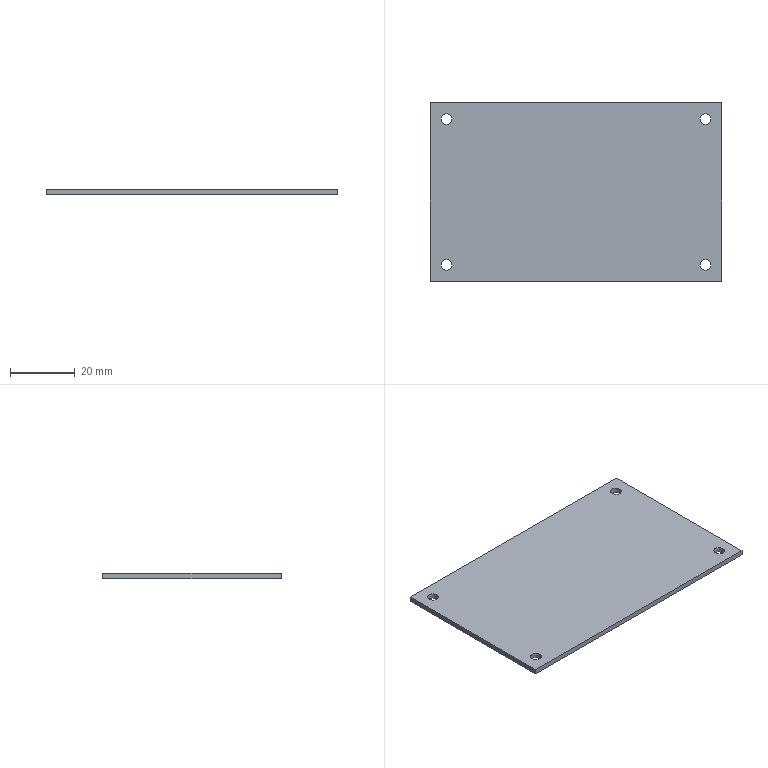Part | SolidWorks | features Extrusion 1 | 1 solid | 14 faces | box 90 x 55 x 1.6 mm | volume 7865 mm3 | cylinder 8 | plane 6 | commonest cylinder face diameters 3.3 x8
STEP:
#1=CARTESIAN_POINT('',(38.35,22.5,-0.8));
#2=VERTEX_POINT('',#1);
#3=CARTESIAN_POINT('',(41.65,22.5,-0.8));
#4=VERTEX_POINT('',#3);
#5=CARTESIAN_POINT('',(40.,22.5,-0.8));
#6=DIRECTION('',(0.,0.,1.));
#7=DIRECTION('',(1.,0.,0.));
#8=AXIS2_PLACEMENT_3D('',#5,#6,#7);
#9=CIRCLE('',#8,1.65);
#10=EDGE_CURVE('',#2,#4,#9,.T.);
#11=ORIENTED_EDGE('',*,*,#10,.F.);
#12=CARTESIAN_POINT('',(38.35,22.5,0.8));
#13=VERTEX_POINT('',#12);
#14=CARTESIAN_POINT('',(38.35,22.5,-0.8));
#15=DIRECTION('',(0.,0.,1.));
#16=VECTOR('',#15,1000.);
#17=LINE('',#14,#16);
#18=EDGE_CURVE('',#2,#13,#17,.T.);
#19=ORIENTED_EDGE('',*,*,#18,.T.);
#20=CARTESIAN_POINT('',(41.65,22.5,0.8));
#21=VERTEX_POINT('',#20);
#22=CARTESIAN_POINT('',(40.,22.5,0.8));
#23=DIRECTION('',(0.,0.,1.));
#24=DIRECTION('',(1.,0.,0.));
#25=AXIS2_PLACEMENT_3D('',#22,#23,#24);
#26=CIRCLE('',#25,1.65);
#27=EDGE_CURVE('',#13,#21,#26,.T.);
#28=ORIENTED_EDGE('',*,*,#27,.T.);
#29=CARTESIAN_POINT('',(41.65,22.5,-0.8));
#30=DIRECTION('',(0.,0.,1.));
#31=VECTOR('',#30,1000.);
#32=LINE('',#29,#31);
#33=EDGE_CURVE('',#4,#21,#32,.T.);
#34=ORIENTED_EDGE('',*,*,#33,.F.);
#35=EDGE_LOOP('',(#11,#19,#28,#34));
#36=FACE_OUTER_BOUND('',#35,.T.);
#37=CARTESIAN_POINT('',(40.,22.5,-0.8));
#38=DIRECTION('',(0.,0.,1.));
#39=DIRECTION('',(1.,0.,0.));
#40=AXIS2_PLACEMENT_3D('',#37,#38,#39);
#41=CYLINDRICAL_SURFACE('',#40,1.65);
#42=ADVANCED_FACE('',(#36),#41,.F.);
#43=CARTESIAN_POINT('',(38.35,-22.5,-0.8));
#44=VERTEX_POINT('',#43);
#45=CARTESIAN_POINT('',(41.65,-22.5,-0.8));
#46=VERTEX_POINT('',#45);
#47=CARTESIAN_POINT('',(40.,-22.5,-0.8));
#48=DIRECTION('',(0.,0.,1.));
#49=DIRECTION('',(1.,0.,0.));
#50=AXIS2_PLACEMENT_3D('',#47,#48,#49);
#51=CIRCLE('',#50,1.65);
#52=EDGE_CURVE('',#44,#46,#51,.T.);
#53=ORIENTED_EDGE('',*,*,#52,.F.);
#54=CARTESIAN_POINT('',(38.35,-22.5,0.8));
#55=VERTEX_POINT('',#54);
#56=CARTESIAN_POINT('',(38.35,-22.5,-0.8));
#57=DIRECTION('',(0.,0.,1.));
#58=VECTOR('',#57,1000.);
#59=LINE('',#56,#58);
#60=EDGE_CURVE('',#44,#55,#59,.T.);
#61=ORIENTED_EDGE('',*,*,#60,.T.);
#62=CARTESIAN_POINT('',(41.65,-22.5,0.8));
#63=VERTEX_POINT('',#62);
#64=CARTESIAN_POINT('',(40.,-22.5,0.8));
#65=DIRECTION('',(0.,0.,1.));
#66=DIRECTION('',(1.,0.,0.));
#67=AXIS2_PLACEMENT_3D('',#64,#65,#66);
#68=CIRCLE('',#67,1.65);
#69=EDGE_CURVE('',#55,#63,#68,.T.);
#70=ORIENTED_EDGE('',*,*,#69,.T.);
#71=CARTESIAN_POINT('',(41.65,-22.5,-0.8));
#72=DIRECTION('',(0.,0.,1.));
#73=VECTOR('',#72,1000.);
#74=LINE('',#71,#73);
#75=EDGE_CURVE('',#46,#63,#74,.T.);
#76=ORIENTED_EDGE('',*,*,#75,.F.);
#77=EDGE_LOOP('',(#53,#61,#70,#76));
#78=FACE_OUTER_BOUND('',#77,.T.);
#79=CARTESIAN_POINT('',(40.,-22.5,-0.8));
#80=DIRECTION('',(0.,0.,1.));
#81=DIRECTION('',(1.,0.,0.));
#82=AXIS2_PLACEMENT_3D('',#79,#80,#81);
#83=CYLINDRICAL_SURFACE('',#82,1.65);
#84=ADVANCED_FACE('',(#78),#83,.F.);
#85=CARTESIAN_POINT('',(-41.65,22.5,-0.8));
#86=VERTEX_POINT('',#85);
#87=CARTESIAN_POINT('',(-38.35,22.5,-0.8));
#88=VERTEX_POINT('',#87);
#89=CARTESIAN_POINT('',(-40.,22.5,-0.8));
#90=DIRECTION('',(0.,0.,1.));
#91=DIRECTION('',(1.,0.,0.));
#92=AXIS2_PLACEMENT_3D('',#89,#90,#91);
#93=CIRCLE('',#92,1.65);
#94=EDGE_CURVE('',#86,#88,#93,.T.);
#95=ORIENTED_EDGE('',*,*,#94,.F.);
#96=CARTESIAN_POINT('',(-41.65,22.5,0.8));
#97=VERTEX_POINT('',#96);
#98=CARTESIAN_POINT('',(-41.65,22.5,-0.8));
#99=DIRECTION('',(0.,0.,1.));
#100=VECTOR('',#99,1000.);
#101=LINE('',#98,#100);
#102=EDGE_CURVE('',#86,#97,#101,.T.);
#103=ORIENTED_EDGE('',*,*,#102,.T.);
#104=CARTESIAN_POINT('',(-38.35,22.5,0.8));
#105=VERTEX_POINT('',#104);
#106=CARTESIAN_POINT('',(-40.,22.5,0.8));
#107=DIRECTION('',(0.,0.,1.));
#108=DIRECTION('',(1.,0.,0.));
#109=AXIS2_PLACEMENT_3D('',#106,#107,#108);
#110=CIRCLE('',#109,1.65);
#111=EDGE_CURVE('',#97,#105,#110,.T.);
#112=ORIENTED_EDGE('',*,*,#111,.T.);
#113=CARTESIAN_POINT('',(-38.35,22.5,-0.8));
#114=DIRECTION('',(0.,0.,1.));
#115=VECTOR('',#114,1000.);
#116=LINE('',#113,#115);
#117=EDGE_CURVE('',#88,#105,#116,.T.);
#118=ORIENTED_EDGE('',*,*,#117,.F.);
#119=EDGE_LOOP('',(#95,#103,#112,#118));
#120=FACE_OUTER_BOUND('',#119,.T.);
#121=CARTESIAN_POINT('',(-40.,22.5,-0.8));
#122=DIRECTION('',(0.,0.,1.));
#123=DIRECTION('',(1.,0.,0.));
#124=AXIS2_PLACEMENT_3D('',#121,#122,#123);
#125=CYLINDRICAL_SURFACE('',#124,1.65);
#126=ADVANCED_FACE('',(#120),#125,.F.);
#127=CARTESIAN_POINT('',(-41.65,-22.5,-0.8));
#128=VERTEX_POINT('',#127);
#129=CARTESIAN_POINT('',(-38.35,-22.5,-0.8));
#130=VERTEX_POINT('',#129);
#131=CARTESIAN_POINT('',(-40.,-22.5,-0.8));
#132=DIRECTION('',(0.,0.,1.));
#133=DIRECTION('',(1.,0.,0.));
#134=AXIS2_PLACEMENT_3D('',#131,#132,#133);
#135=CIRCLE('',#134,1.65);
#136=EDGE_CURVE('',#128,#130,#135,.T.);
#137=ORIENTED_EDGE('',*,*,#136,.F.);
#138=CARTESIAN_POINT('',(-41.65,-22.5,0.8));
#139=VERTEX_POINT('',#138);
#140=CARTESIAN_POINT('',(-41.65,-22.5,-0.8));
#141=DIRECTION('',(0.,0.,1.));
#142=VECTOR('',#141,1000.);
#143=LINE('',#140,#142);
#144=EDGE_CURVE('',#128,#139,#143,.T.);
#145=ORIENTED_EDGE('',*,*,#144,.T.);
#146=CARTESIAN_POINT('',(-38.35,-22.5,0.8));
#147=VERTEX_POINT('',#146);
#148=CARTESIAN_POINT('',(-40.,-22.5,0.8));
#149=DIRECTION('',(0.,0.,1.));
#150=DIRECTION('',(1.,0.,0.));
#151=AXIS2_PLACEMENT_3D('',#148,#149,#150);
#152=CIRCLE('',#151,1.65);
#153=EDGE_CURVE('',#139,#147,#152,.T.);
#154=ORIENTED_EDGE('',*,*,#153,.T.);
#155=CARTESIAN_POINT('',(-38.35,-22.5,-0.8));
#156=DIRECTION('',(0.,0.,1.));
#157=VECTOR('',#156,1000.);
#158=LINE('',#155,#157);
#159=EDGE_CURVE('',#130,#147,#158,.T.);
#160=ORIENTED_EDGE('',*,*,#159,.F.);
#161=EDGE_LOOP('',(#137,#145,#154,#160));
#162=FACE_OUTER_BOUND('',#161,.T.);
#163=CARTESIAN_POINT('',(-40.,-22.5,-0.8));
#164=DIRECTION('',(0.,0.,1.));
#165=DIRECTION('',(1.,0.,0.));
#166=AXIS2_PLACEMENT_3D('',#163,#164,#165);
#167=CYLINDRICAL_SURFACE('',#166,1.65);
#168=ADVANCED_FACE('',(#162),#167,.F.);
#169=CARTESIAN_POINT('',(-45.,27.5,0.8));
#170=VERTEX_POINT('',#169);
#171=CARTESIAN_POINT('',(-45.,-27.5,0.8));
#172=VERTEX_POINT('',#171);
#173=CARTESIAN_POINT('',(-45.,27.5,0.8));
#174=DIRECTION('',(0.,-1.,0.));
#175=VECTOR('',#174,1000.);
#176=LINE('',#173,#175);
#177=EDGE_CURVE('',#170,#172,#176,.T.);
#178=ORIENTED_EDGE('',*,*,#177,.F.);
#179=CARTESIAN_POINT('',(-45.,27.5,-0.8));
#180=VERTEX_POINT('',#179);
#181=CARTESIAN_POINT('',(-45.,27.5,-0.8));
#182=DIRECTION('',(0.,0.,1.));
#183=VECTOR('',#182,1000.);
#184=LINE('',#181,#183);
#185=EDGE_CURVE('',#180,#170,#184,.T.);
#186=ORIENTED_EDGE('',*,*,#185,.F.);
#187=CARTESIAN_POINT('',(-45.,-27.5,-0.8));
#188=VERTEX_POINT('',#187);
#189=CARTESIAN_POINT('',(-45.,27.5,-0.8));
#190=DIRECTION('',(0.,-1.,0.));
#191=VECTOR('',#190,1000.);
#192=LINE('',#189,#191);
#193=EDGE_CURVE('',#180,#188,#192,.T.);
#194=ORIENTED_EDGE('',*,*,#193,.T.);
#195=CARTESIAN_POINT('',(-45.,-27.5,-0.8));
#196=DIRECTION('',(0.,0.,1.));
#197=VECTOR('',#196,1000.);
#198=LINE('',#195,#197);
#199=EDGE_CURVE('',#188,#172,#198,.T.);
#200=ORIENTED_EDGE('',*,*,#199,.T.);
#201=EDGE_LOOP('',(#178,#186,#194,#200));
#202=FACE_OUTER_BOUND('',#201,.T.);
#203=CARTESIAN_POINT('',(-45.,27.5,-0.8));
#204=DIRECTION('',(-1.,0.,0.));
#205=DIRECTION('',(0.,0.,1.));
#206=AXIS2_PLACEMENT_3D('',#203,#204,#205);
#207=PLANE('',#206);
#208=ADVANCED_FACE('',(#202),#207,.T.);
#209=CARTESIAN_POINT('',(45.,27.5,0.8));
#210=VERTEX_POINT('',#209);
#211=CARTESIAN_POINT('',(45.,27.5,0.8));
#212=DIRECTION('',(-1.,0.,0.));
#213=VECTOR('',#212,1000.);
#214=LINE('',#211,#213);
#215=EDGE_CURVE('',#210,#170,#214,.T.);
#216=ORIENTED_EDGE('',*,*,#215,.F.);
#217=CARTESIAN_POINT('',(45.,27.5,-0.8));
#218=VERTEX_POINT('',#217);
#219=CARTESIAN_POINT('',(45.,27.5,-0.8));
#220=DIRECTION('',(0.,0.,1.));
#221=VECTOR('',#220,1000.);
#222=LINE('',#219,#221);
#223=EDGE_CURVE('',#218,#210,#222,.T.);
#224=ORIENTED_EDGE('',*,*,#223,.F.);
#225=CARTESIAN_POINT('',(45.,27.5,-0.8));
#226=DIRECTION('',(-1.,0.,0.));
#227=VECTOR('',#226,1000.);
#228=LINE('',#225,#227);
#229=EDGE_CURVE('',#218,#180,#228,.T.);
#230=ORIENTED_EDGE('',*,*,#229,.T.);
#231=ORIENTED_EDGE('',*,*,#185,.T.);
#232=EDGE_LOOP('',(#216,#224,#230,#231));
#233=FACE_OUTER_BOUND('',#232,.T.);
#234=CARTESIAN_POINT('',(45.,27.5,-0.8));
#235=DIRECTION('',(0.,1.,0.));
#236=DIRECTION('',(0.,0.,1.));
#237=AXIS2_PLACEMENT_3D('',#234,#235,#236);
#238=PLANE('',#237);
#239=ADVANCED_FACE('',(#233),#238,.T.);
#240=CARTESIAN_POINT('',(45.,-27.5,0.8));
#241=VERTEX_POINT('',#240);
#242=CARTESIAN_POINT('',(45.,-27.5,0.8));
#243=DIRECTION('',(0.,1.,0.));
#244=VECTOR('',#243,1000.);
#245=LINE('',#242,#244);
#246=EDGE_CURVE('',#241,#210,#245,.T.);
#247=ORIENTED_EDGE('',*,*,#246,.F.);
#248=CARTESIAN_POINT('',(45.,-27.5,-0.8));
#249=VERTEX_POINT('',#248);
#250=CARTESIAN_POINT('',(45.,-27.5,-0.8));
#251=DIRECTION('',(0.,0.,1.));
#252=VECTOR('',#251,1000.);
#253=LINE('',#250,#252);
#254=EDGE_CURVE('',#249,#241,#253,.T.);
#255=ORIENTED_EDGE('',*,*,#254,.F.);
#256=CARTESIAN_POINT('',(45.,-27.5,-0.8));
#257=DIRECTION('',(0.,1.,0.));
#258=VECTOR('',#257,1000.);
#259=LINE('',#256,#258);
#260=EDGE_CURVE('',#249,#218,#259,.T.);
#261=ORIENTED_EDGE('',*,*,#260,.T.);
#262=ORIENTED_EDGE('',*,*,#223,.T.);
#263=EDGE_LOOP('',(#247,#255,#261,#262));
#264=FACE_OUTER_BOUND('',#263,.T.);
#265=CARTESIAN_POINT('',(45.,-27.5,-0.8));
#266=DIRECTION('',(1.,0.,0.));
#267=DIRECTION('',(0.,0.,-1.));
#268=AXIS2_PLACEMENT_3D('',#265,#266,#267);
#269=PLANE('',#268);
#270=ADVANCED_FACE('',(#264),#269,.T.);
#271=CARTESIAN_POINT('',(-45.,-27.5,0.8));
#272=DIRECTION('',(1.,0.,0.));
#273=VECTOR('',#272,1000.);
#274=LINE('',#271,#273);
#275=EDGE_CURVE('',#172,#241,#274,.T.);
#276=ORIENTED_EDGE('',*,*,#275,.F.);
#277=ORIENTED_EDGE('',*,*,#199,.F.);
#278=CARTESIAN_POINT('',(-45.,-27.5,-0.8));
#279=DIRECTION('',(1.,0.,0.));
#280=VECTOR('',#279,1000.);
#281=LINE('',#278,#280);
#282=EDGE_CURVE('',#188,#249,#281,.T.);
#283=ORIENTED_EDGE('',*,*,#282,.T.);
#284=ORIENTED_EDGE('',*,*,#254,.T.);
#285=EDGE_LOOP('',(#276,#277,#283,#284));
#286=FACE_OUTER_BOUND('',#285,.T.);
#287=CARTESIAN_POINT('',(-45.,-27.5,-0.8));
#288=DIRECTION('',(0.,-1.,0.));
#289=DIRECTION('',(0.,0.,-1.));
#290=AXIS2_PLACEMENT_3D('',#287,#288,#289);
#291=PLANE('',#290);
#292=ADVANCED_FACE('',(#286),#291,.T.);
#293=CARTESIAN_POINT('',(40.,22.5,-0.8));
#294=DIRECTION('',(0.,0.,1.));
#295=DIRECTION('',(1.,0.,0.));
#296=AXIS2_PLACEMENT_3D('',#293,#294,#295);
#297=CIRCLE('',#296,1.65);
#298=EDGE_CURVE('',#4,#2,#297,.T.);
#299=ORIENTED_EDGE('',*,*,#298,.T.);
#300=ORIENTED_EDGE('',*,*,#10,.T.);
#301=EDGE_LOOP('',(#299,#300));
#302=FACE_BOUND('',#301,.T.);
#303=CARTESIAN_POINT('',(40.,-22.5,-0.8));
#304=DIRECTION('',(0.,0.,1.));
#305=DIRECTION('',(1.,0.,0.));
#306=AXIS2_PLACEMENT_3D('',#303,#304,#305);
#307=CIRCLE('',#306,1.65);
#308=EDGE_CURVE('',#46,#44,#307,.T.);
#309=ORIENTED_EDGE('',*,*,#308,.T.);
#310=ORIENTED_EDGE('',*,*,#52,.T.);
#311=EDGE_LOOP('',(#309,#310));
#312=FACE_BOUND('',#311,.T.);
#313=CARTESIAN_POINT('',(-40.,22.5,-0.8));
#314=DIRECTION('',(0.,0.,1.));
#315=DIRECTION('',(1.,0.,0.));
#316=AXIS2_PLACEMENT_3D('',#313,#314,#315);
#317=CIRCLE('',#316,1.65);
#318=EDGE_CURVE('',#88,#86,#317,.T.);
#319=ORIENTED_EDGE('',*,*,#318,.T.);
#320=ORIENTED_EDGE('',*,*,#94,.T.);
#321=EDGE_LOOP('',(#319,#320));
#322=FACE_BOUND('',#321,.T.);
#323=CARTESIAN_POINT('',(-40.,-22.5,-0.8));
#324=DIRECTION('',(0.,0.,1.));
#325=DIRECTION('',(1.,0.,0.));
#326=AXIS2_PLACEMENT_3D('',#323,#324,#325);
#327=CIRCLE('',#326,1.65);
#328=EDGE_CURVE('',#130,#128,#327,.T.);
#329=ORIENTED_EDGE('',*,*,#328,.T.);
#330=ORIENTED_EDGE('',*,*,#136,.T.);
#331=EDGE_LOOP('',(#329,#330));
#332=FACE_BOUND('',#331,.T.);
#333=ORIENTED_EDGE('',*,*,#193,.F.);
#334=ORIENTED_EDGE('',*,*,#229,.F.);
#335=ORIENTED_EDGE('',*,*,#260,.F.);
#336=ORIENTED_EDGE('',*,*,#282,.F.);
#337=EDGE_LOOP('',(#333,#334,#335,#336));
#338=FACE_OUTER_BOUND('',#337,.T.);
#339=CARTESIAN_POINT('',(0.,0.,-0.8));
#340=DIRECTION('',(0.,0.,1.));
#341=DIRECTION('',(1.,0.,0.));
#342=AXIS2_PLACEMENT_3D('',#339,#340,#341);
#343=PLANE('',#342);
#344=ADVANCED_FACE('',(#302,#312,#322,#332,#338),#343,.F.);
#345=CARTESIAN_POINT('',(40.,22.5,0.8));
#346=DIRECTION('',(0.,0.,1.));
#347=DIRECTION('',(1.,0.,0.));
#348=AXIS2_PLACEMENT_3D('',#345,#346,#347);
#349=CIRCLE('',#348,1.65);
#350=EDGE_CURVE('',#21,#13,#349,.T.);
#351=ORIENTED_EDGE('',*,*,#350,.F.);
#352=ORIENTED_EDGE('',*,*,#27,.F.);
#353=EDGE_LOOP('',(#351,#352));
#354=FACE_BOUND('',#353,.T.);
#355=CARTESIAN_POINT('',(40.,-22.5,0.8));
#356=DIRECTION('',(0.,0.,1.));
#357=DIRECTION('',(1.,0.,0.));
#358=AXIS2_PLACEMENT_3D('',#355,#356,#357);
#359=CIRCLE('',#358,1.65);
#360=EDGE_CURVE('',#63,#55,#359,.T.);
#361=ORIENTED_EDGE('',*,*,#360,.F.);
#362=ORIENTED_EDGE('',*,*,#69,.F.);
#363=EDGE_LOOP('',(#361,#362));
#364=FACE_BOUND('',#363,.T.);
#365=CARTESIAN_POINT('',(-40.,22.5,0.8));
#366=DIRECTION('',(0.,0.,1.));
#367=DIRECTION('',(1.,0.,0.));
#368=AXIS2_PLACEMENT_3D('',#365,#366,#367);
#369=CIRCLE('',#368,1.65);
#370=EDGE_CURVE('',#105,#97,#369,.T.);
#371=ORIENTED_EDGE('',*,*,#370,.F.);
#372=ORIENTED_EDGE('',*,*,#111,.F.);
#373=EDGE_LOOP('',(#371,#372));
#374=FACE_BOUND('',#373,.T.);
#375=CARTESIAN_POINT('',(-40.,-22.5,0.8));
#376=DIRECTION('',(0.,0.,1.));
#377=DIRECTION('',(1.,0.,0.));
#378=AXIS2_PLACEMENT_3D('',#375,#376,#377);
#379=CIRCLE('',#378,1.65);
#380=EDGE_CURVE('',#147,#139,#379,.T.);
#381=ORIENTED_EDGE('',*,*,#380,.F.);
#382=ORIENTED_EDGE('',*,*,#153,.F.);
#383=EDGE_LOOP('',(#381,#382));
#384=FACE_BOUND('',#383,.T.);
#385=ORIENTED_EDGE('',*,*,#177,.T.);
#386=ORIENTED_EDGE('',*,*,#275,.T.);
#387=ORIENTED_EDGE('',*,*,#246,.T.);
#388=ORIENTED_EDGE('',*,*,#215,.T.);
#389=EDGE_LOOP('',(#385,#386,#387,#388));
#390=FACE_OUTER_BOUND('',#389,.T.);
#391=CARTESIAN_POINT('',(0.,0.,0.8));
#392=DIRECTION('',(0.,0.,1.));
#393=DIRECTION('',(1.,0.,0.));
#394=AXIS2_PLACEMENT_3D('',#391,#392,#393);
#395=PLANE('',#394);
#396=ADVANCED_FACE('',(#354,#364,#374,#384,#390),#395,.T.);
#397=ORIENTED_EDGE('',*,*,#144,.F.);
#398=ORIENTED_EDGE('',*,*,#328,.F.);
#399=ORIENTED_EDGE('',*,*,#159,.T.);
#400=ORIENTED_EDGE('',*,*,#380,.T.);
#401=EDGE_LOOP('',(#397,#398,#399,#400));
#402=FACE_OUTER_BOUND('',#401,.T.);
#403=CARTESIAN_POINT('',(-40.,-22.5,-0.8));
#404=DIRECTION('',(0.,0.,1.));
#405=DIRECTION('',(1.,0.,0.));
#406=AXIS2_PLACEMENT_3D('',#403,#404,#405);
#407=CYLINDRICAL_SURFACE('',#406,1.65);
#408=ADVANCED_FACE('',(#402),#407,.F.);
#409=ORIENTED_EDGE('',*,*,#102,.F.);
#410=ORIENTED_EDGE('',*,*,#318,.F.);
#411=ORIENTED_EDGE('',*,*,#117,.T.);
#412=ORIENTED_EDGE('',*,*,#370,.T.);
#413=EDGE_LOOP('',(#409,#410,#411,#412));
#414=FACE_OUTER_BOUND('',#413,.T.);
#415=CARTESIAN_POINT('',(-40.,22.5,-0.8));
#416=DIRECTION('',(0.,0.,1.));
#417=DIRECTION('',(1.,0.,0.));
#418=AXIS2_PLACEMENT_3D('',#415,#416,#417);
#419=CYLINDRICAL_SURFACE('',#418,1.65);
#420=ADVANCED_FACE('',(#414),#419,.F.);
#421=ORIENTED_EDGE('',*,*,#60,.F.);
#422=ORIENTED_EDGE('',*,*,#308,.F.);
#423=ORIENTED_EDGE('',*,*,#75,.T.);
#424=ORIENTED_EDGE('',*,*,#360,.T.);
#425=EDGE_LOOP('',(#421,#422,#423,#424));
#426=FACE_OUTER_BOUND('',#425,.T.);
#427=CARTESIAN_POINT('',(40.,-22.5,-0.8));
#428=DIRECTION('',(0.,0.,1.));
#429=DIRECTION('',(1.,0.,0.));
#430=AXIS2_PLACEMENT_3D('',#427,#428,#429);
#431=CYLINDRICAL_SURFACE('',#430,1.65);
#432=ADVANCED_FACE('',(#426),#431,.F.);
#433=ORIENTED_EDGE('',*,*,#18,.F.);
#434=ORIENTED_EDGE('',*,*,#298,.F.);
#435=ORIENTED_EDGE('',*,*,#33,.T.);
#436=ORIENTED_EDGE('',*,*,#350,.T.);
#437=EDGE_LOOP('',(#433,#434,#435,#436));
#438=FACE_OUTER_BOUND('',#437,.T.);
#439=CARTESIAN_POINT('',(40.,22.5,-0.8));
#440=DIRECTION('',(0.,0.,1.));
#441=DIRECTION('',(1.,0.,0.));
#442=AXIS2_PLACEMENT_3D('',#439,#440,#441);
#443=CYLINDRICAL_SURFACE('',#442,1.65);
#444=ADVANCED_FACE('',(#438),#443,.F.);
#445=CLOSED_SHELL('',(#42,#84,#126,#168,#208,#239,#270,#292,#344,#396,#408,#420,#432,#444));
#446=MANIFOLD_SOLID_BREP('',#445);
#447=CARTESIAN_POINT('',(0.,0.,0.));
#448=DIRECTION('',(0.,0.,1.));
#449=DIRECTION('',(1.,0.,0.));
#450=AXIS2_PLACEMENT_3D('',#447,#448,#449);
#451=(LENGTH_UNIT()NAMED_UNIT(*)SI_UNIT(.MILLI.,.METRE.));
#452=UNCERTAINTY_MEASURE_WITH_UNIT(LENGTH_MEASURE(0.00001),#451,'','');
#453=(NAMED_UNIT(*)PLANE_ANGLE_UNIT()SI_UNIT($,.RADIAN.));
#454=(NAMED_UNIT(*)SI_UNIT($,.STERADIAN.)SOLID_ANGLE_UNIT());
#455=(GEOMETRIC_REPRESENTATION_CONTEXT(3)GLOBAL_UNCERTAINTY_ASSIGNED_CONTEXT((#452))GLOBAL_UNIT_ASSIGNED_CONTEXT((#451,#453,#454))REPRESENTATION_CONTEXT('',''));
#456=ADVANCED_BREP_SHAPE_REPRESENTATION('',(#446,#450),#455);